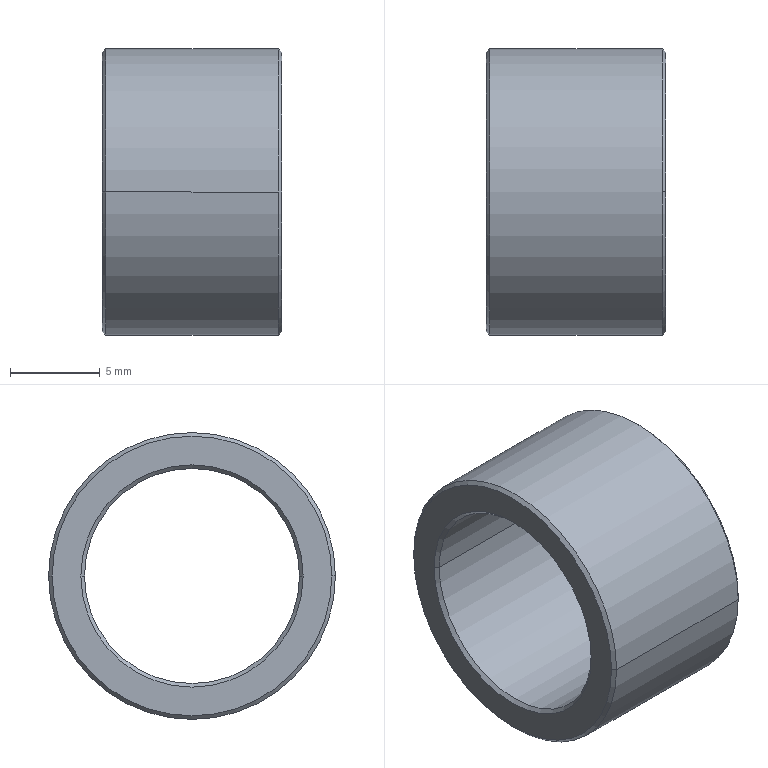Part | STEP file | 0230_009_KNCLB12-16-10 | 1 solid | 14 faces | box 10 x 16 x 16 mm | volume 876.127 mm3 | cone 8 | cylinder 4 | plane 2 | commonest cylinder face diameters 12 x2 16 x2
STEP:
#1=CARTESIAN_POINT('',(0.,0.,0.));
#2=DIRECTION('',(0.,0.,1.));
#3=DIRECTION('',(1.,0.,0.));
#4=AXIS2_PLACEMENT_3D('',#1,#2,#3);
#5=CARTESIAN_POINT('',(9.8,0.,8.));
#6=VERTEX_POINT('',#5);
#7=CARTESIAN_POINT('',(9.8,8.,0.));
#8=VERTEX_POINT('',#7);
#9=CARTESIAN_POINT('',(9.8,0.,0.));
#10=DIRECTION('',(-1.,0.,0.));
#11=DIRECTION('',(0.,-1.,0.));
#12=AXIS2_PLACEMENT_3D('',#9,#10,#11);
#13=CIRCLE('',#12,8.);
#14=CARTESIAN_POINT('',(5.,0.,0.));
#15=DIRECTION('',(-1.,0.,0.));
#16=DIRECTION('',(0.,-1.,0.));
#17=AXIS2_PLACEMENT_3D('',#14,#15,#16);
#18=CYLINDRICAL_SURFACE('',#17,8.);
#19=CARTESIAN_POINT('',(0.,-4.8));
#20=DIRECTION('',(1.,0.));
#21=VECTOR('',#20,1.);
#22=LINE('',#19,#21);
#23=(GEOMETRIC_REPRESENTATION_CONTEXT(2)PARAMETRIC_REPRESENTATION_CONTEXT()REPRESENTATION_CONTEXT('',''));
#24=DEFINITIONAL_REPRESENTATION('',(#22),#23);
#25=PCURVE('',#18,#24);
#26=CARTESIAN_POINT('',(9.8,0.,0.));
#27=DIRECTION('',(-1.,0.,0.));
#28=DIRECTION('',(0.,0.,1.));
#29=AXIS2_PLACEMENT_3D('',#26,#27,#28);
#30=CONICAL_SURFACE('',#29,8.,0.7854);
#31=CARTESIAN_POINT('',(-1.571,0.));
#32=DIRECTION('',(1.,0.));
#33=VECTOR('',#32,1.);
#34=LINE('',#31,#33);
#35=(GEOMETRIC_REPRESENTATION_CONTEXT(2)PARAMETRIC_REPRESENTATION_CONTEXT()REPRESENTATION_CONTEXT('',''));
#36=DEFINITIONAL_REPRESENTATION('',(#34),#35);
#37=PCURVE('',#30,#36);
#38=SURFACE_CURVE('',#13,(#25,#37),.PCURVE_S1.);
#39=EDGE_CURVE('',#6,#8,#38,.T.);
#40=ORIENTED_EDGE('',*,*,#39,.T.);
#41=CARTESIAN_POINT('',(0.2,8.,0.));
#42=VERTEX_POINT('',#41);
#43=CARTESIAN_POINT('',(5.,8.,0.));
#44=DIRECTION('',(-1.,0.,0.));
#45=VECTOR('',#44,1.);
#46=LINE('',#43,#45);
#47=CARTESIAN_POINT('',(3.142,0.));
#48=DIRECTION('',(0.,1.));
#49=VECTOR('',#48,1.);
#50=LINE('',#47,#49);
#51=(GEOMETRIC_REPRESENTATION_CONTEXT(2)PARAMETRIC_REPRESENTATION_CONTEXT()REPRESENTATION_CONTEXT('',''));
#52=DEFINITIONAL_REPRESENTATION('',(#50),#51);
#53=PCURVE('',#18,#52);
#54=CARTESIAN_POINT('',(5.,0.,0.));
#55=DIRECTION('',(-1.,0.,0.));
#56=DIRECTION('',(0.,-1.,0.));
#57=AXIS2_PLACEMENT_3D('',#54,#55,#56);
#58=CYLINDRICAL_SURFACE('',#57,8.);
#59=CARTESIAN_POINT('',(3.142,0.));
#60=DIRECTION('',(0.,1.));
#61=VECTOR('',#60,1.);
#62=LINE('',#59,#61);
#63=(GEOMETRIC_REPRESENTATION_CONTEXT(2)PARAMETRIC_REPRESENTATION_CONTEXT()REPRESENTATION_CONTEXT('',''));
#64=DEFINITIONAL_REPRESENTATION('',(#62),#63);
#65=PCURVE('',#58,#64);
#66=SURFACE_CURVE('',#46,(#53,#65),.PCURVE_S1.);
#67=EDGE_CURVE('',#8,#42,#66,.T.);
#68=ORIENTED_EDGE('',*,*,#67,.T.);
#69=CARTESIAN_POINT('',(0.2,-8.,0.));
#70=VERTEX_POINT('',#69);
#71=CARTESIAN_POINT('',(0.2,0.,0.));
#72=DIRECTION('',(1.,0.,0.));
#73=DIRECTION('',(0.,-1.,0.));
#74=AXIS2_PLACEMENT_3D('',#71,#72,#73);
#75=CIRCLE('',#74,8.);
#76=CARTESIAN_POINT('',(6.283,4.8));
#77=DIRECTION('',(-1.,0.));
#78=VECTOR('',#77,1.);
#79=LINE('',#76,#78);
#80=(GEOMETRIC_REPRESENTATION_CONTEXT(2)PARAMETRIC_REPRESENTATION_CONTEXT()REPRESENTATION_CONTEXT('',''));
#81=DEFINITIONAL_REPRESENTATION('',(#79),#80);
#82=PCURVE('',#18,#81);
#83=CARTESIAN_POINT('',(0.2,0.,0.));
#84=DIRECTION('',(1.,0.,0.));
#85=DIRECTION('',(0.,1.,0.));
#86=AXIS2_PLACEMENT_3D('',#83,#84,#85);
#87=CONICAL_SURFACE('',#86,8.,0.7854);
#88=CARTESIAN_POINT('',(-3.142,0.));
#89=DIRECTION('',(1.,0.));
#90=VECTOR('',#89,1.);
#91=LINE('',#88,#90);
#92=(GEOMETRIC_REPRESENTATION_CONTEXT(2)PARAMETRIC_REPRESENTATION_CONTEXT()REPRESENTATION_CONTEXT('',''));
#93=DEFINITIONAL_REPRESENTATION('',(#91),#92);
#94=PCURVE('',#87,#93);
#95=SURFACE_CURVE('',#75,(#82,#94),.PCURVE_S1.);
#96=EDGE_CURVE('',#42,#70,#95,.T.);
#97=ORIENTED_EDGE('',*,*,#96,.T.);
#98=CARTESIAN_POINT('',(9.8,-8.,0.));
#99=VERTEX_POINT('',#98);
#100=CARTESIAN_POINT('',(5.,-8.,0.));
#101=DIRECTION('',(-1.,0.,0.));
#102=VECTOR('',#101,1.);
#103=LINE('',#100,#102);
#104=CARTESIAN_POINT('',(0.,0.));
#105=DIRECTION('',(0.,1.));
#106=VECTOR('',#105,1.);
#107=LINE('',#104,#106);
#108=(GEOMETRIC_REPRESENTATION_CONTEXT(2)PARAMETRIC_REPRESENTATION_CONTEXT()REPRESENTATION_CONTEXT('',''));
#109=DEFINITIONAL_REPRESENTATION('',(#107),#108);
#110=PCURVE('',#18,#109);
#111=CARTESIAN_POINT('',(6.283,0.));
#112=DIRECTION('',(0.,1.));
#113=VECTOR('',#112,1.);
#114=LINE('',#111,#113);
#115=(GEOMETRIC_REPRESENTATION_CONTEXT(2)PARAMETRIC_REPRESENTATION_CONTEXT()REPRESENTATION_CONTEXT('',''));
#116=DEFINITIONAL_REPRESENTATION('',(#114),#115);
#117=PCURVE('',#58,#116);
#118=SURFACE_CURVE('',#103,(#110,#117),.PCURVE_S1.);
#119=EDGE_CURVE('',#99,#70,#118,.T.);
#120=ORIENTED_EDGE('',*,*,#119,.F.);
#121=CARTESIAN_POINT('',(9.8,0.,0.));
#122=DIRECTION('',(-1.,0.,0.));
#123=DIRECTION('',(0.,-1.,0.));
#124=AXIS2_PLACEMENT_3D('',#121,#122,#123);
#125=CIRCLE('',#124,8.);
#126=CARTESIAN_POINT('',(0.,-4.8));
#127=DIRECTION('',(1.,0.));
#128=VECTOR('',#127,1.);
#129=LINE('',#126,#128);
#130=(GEOMETRIC_REPRESENTATION_CONTEXT(2)PARAMETRIC_REPRESENTATION_CONTEXT()REPRESENTATION_CONTEXT('',''));
#131=DEFINITIONAL_REPRESENTATION('',(#129),#130);
#132=PCURVE('',#18,#131);
#133=CARTESIAN_POINT('',(9.8,0.,0.));
#134=DIRECTION('',(-1.,0.,0.));
#135=DIRECTION('',(0.,0.,1.));
#136=AXIS2_PLACEMENT_3D('',#133,#134,#135);
#137=CONICAL_SURFACE('',#136,8.,0.7854);
#138=CARTESIAN_POINT('',(4.712,0.));
#139=DIRECTION('',(1.,0.));
#140=VECTOR('',#139,1.);
#141=LINE('',#138,#140);
#142=(GEOMETRIC_REPRESENTATION_CONTEXT(2)PARAMETRIC_REPRESENTATION_CONTEXT()REPRESENTATION_CONTEXT('',''));
#143=DEFINITIONAL_REPRESENTATION('',(#141),#142);
#144=PCURVE('',#137,#143);
#145=SURFACE_CURVE('',#125,(#132,#144),.PCURVE_S1.);
#146=EDGE_CURVE('',#99,#6,#145,.T.);
#147=ORIENTED_EDGE('',*,*,#146,.T.);
#148=EDGE_LOOP('',(#40,#68,#97,#120,#147));
#149=FACE_BOUND('',#148,.T.);
#150=ADVANCED_FACE('',(#149),#18,.T.);
#151=CARTESIAN_POINT('',(10.,0.,7.8));
#152=VERTEX_POINT('',#151);
#153=CARTESIAN_POINT('',(10.,0.,-7.8));
#154=VERTEX_POINT('',#153);
#155=CARTESIAN_POINT('',(10.,0.,0.));
#156=DIRECTION('',(-1.,0.,0.));
#157=DIRECTION('',(0.,0.,1.));
#158=AXIS2_PLACEMENT_3D('',#155,#156,#157);
#159=CIRCLE('',#158,7.8);
#160=CARTESIAN_POINT('',(0.,-0.2));
#161=DIRECTION('',(1.,0.));
#162=VECTOR('',#161,1.);
#163=LINE('',#160,#162);
#164=(GEOMETRIC_REPRESENTATION_CONTEXT(2)PARAMETRIC_REPRESENTATION_CONTEXT()REPRESENTATION_CONTEXT('',''));
#165=DEFINITIONAL_REPRESENTATION('',(#163),#164);
#166=PCURVE('',#30,#165);
#167=CARTESIAN_POINT('',(10.,-7.,0.));
#168=DIRECTION('',(1.,0.,0.));
#169=DIRECTION('',(0.,0.,-1.));
#170=AXIS2_PLACEMENT_3D('',#167,#168,#169);
#171=PLANE('',#170);
#172=CARTESIAN_POINT('',(-7.8,7.));
#173=CARTESIAN_POINT('',(-7.8,20.51));
#174=CARTESIAN_POINT('',(3.9,13.755));
#175=CARTESIAN_POINT('',(15.6,7.));
#176=CARTESIAN_POINT('',(3.9,0.245));
#177=CARTESIAN_POINT('',(-7.8,-6.51));
#178=CARTESIAN_POINT('',(-7.8,7.));
#179=(BOUNDED_CURVE()B_SPLINE_CURVE(2,(#172,#173,#174,#175,#176,#177,#178),.UNSPECIFIED.,.T.,.F.)B_SPLINE_CURVE_WITH_KNOTS((1,2,2,2,2,1),(-2.094,0.,2.094,4.189,6.283,8.378),.UNSPECIFIED.)CURVE()GEOMETRIC_REPRESENTATION_ITEM()RATIONAL_B_SPLINE_CURVE((1.,0.5,1.,0.5,1.,0.5,1.))REPRESENTATION_ITEM(''));
#180=(GEOMETRIC_REPRESENTATION_CONTEXT(2)PARAMETRIC_REPRESENTATION_CONTEXT()REPRESENTATION_CONTEXT('',''));
#181=DEFINITIONAL_REPRESENTATION('',(#179),#180);
#182=PCURVE('',#171,#181);
#183=SURFACE_CURVE('',#159,(#166,#182),.PCURVE_S1.);
#184=EDGE_CURVE('',#152,#154,#183,.T.);
#185=ORIENTED_EDGE('',*,*,#184,.T.);
#186=CARTESIAN_POINT('',(9.8,0.,-8.));
#187=VERTEX_POINT('',#186);
#188=CARTESIAN_POINT('',(9.8,0.,-8.));
#189=DIRECTION('',(-0.7071,0.,-0.7071));
#190=VECTOR('',#189,1.);
#191=LINE('',#188,#190);
#192=CARTESIAN_POINT('',(3.142,0.));
#193=DIRECTION('',(0.,1.));
#194=VECTOR('',#193,1.);
#195=LINE('',#192,#194);
#196=(GEOMETRIC_REPRESENTATION_CONTEXT(2)PARAMETRIC_REPRESENTATION_CONTEXT()REPRESENTATION_CONTEXT('',''));
#197=DEFINITIONAL_REPRESENTATION('',(#195),#196);
#198=PCURVE('',#30,#197);
#199=CARTESIAN_POINT('',(3.142,0.));
#200=DIRECTION('',(0.,1.));
#201=VECTOR('',#200,1.);
#202=LINE('',#199,#201);
#203=(GEOMETRIC_REPRESENTATION_CONTEXT(2)PARAMETRIC_REPRESENTATION_CONTEXT()REPRESENTATION_CONTEXT('',''));
#204=DEFINITIONAL_REPRESENTATION('',(#202),#203);
#205=PCURVE('',#137,#204);
#206=SURFACE_CURVE('',#191,(#198,#205),.PCURVE_S1.);
#207=EDGE_CURVE('',#154,#187,#206,.T.);
#208=ORIENTED_EDGE('',*,*,#207,.T.);
#209=CARTESIAN_POINT('',(9.8,0.,0.));
#210=DIRECTION('',(-1.,0.,0.));
#211=DIRECTION('',(0.,-1.,0.));
#212=AXIS2_PLACEMENT_3D('',#209,#210,#211);
#213=CIRCLE('',#212,8.);
#214=CARTESIAN_POINT('',(-1.571,0.));
#215=DIRECTION('',(1.,0.));
#216=VECTOR('',#215,1.);
#217=LINE('',#214,#216);
#218=(GEOMETRIC_REPRESENTATION_CONTEXT(2)PARAMETRIC_REPRESENTATION_CONTEXT()REPRESENTATION_CONTEXT('',''));
#219=DEFINITIONAL_REPRESENTATION('',(#217),#218);
#220=PCURVE('',#30,#219);
#221=CARTESIAN_POINT('',(0.,-4.8));
#222=DIRECTION('',(1.,0.));
#223=VECTOR('',#222,1.);
#224=LINE('',#221,#223);
#225=(GEOMETRIC_REPRESENTATION_CONTEXT(2)PARAMETRIC_REPRESENTATION_CONTEXT()REPRESENTATION_CONTEXT('',''));
#226=DEFINITIONAL_REPRESENTATION('',(#224),#225);
#227=PCURVE('',#58,#226);
#228=SURFACE_CURVE('',#213,(#220,#227),.PCURVE_S1.);
#229=EDGE_CURVE('',#8,#187,#228,.T.);
#230=ORIENTED_EDGE('',*,*,#229,.F.);
#231=ORIENTED_EDGE('',*,*,#39,.F.);
#232=CARTESIAN_POINT('',(9.8,0.,8.));
#233=DIRECTION('',(-0.7071,0.,0.7071));
#234=VECTOR('',#233,1.);
#235=LINE('',#232,#234);
#236=CARTESIAN_POINT('',(0.,0.));
#237=DIRECTION('',(0.,1.));
#238=VECTOR('',#237,1.);
#239=LINE('',#236,#238);
#240=(GEOMETRIC_REPRESENTATION_CONTEXT(2)PARAMETRIC_REPRESENTATION_CONTEXT()REPRESENTATION_CONTEXT('',''));
#241=DEFINITIONAL_REPRESENTATION('',(#239),#240);
#242=PCURVE('',#30,#241);
#243=CARTESIAN_POINT('',(6.283,0.));
#244=DIRECTION('',(0.,1.));
#245=VECTOR('',#244,1.);
#246=LINE('',#243,#245);
#247=(GEOMETRIC_REPRESENTATION_CONTEXT(2)PARAMETRIC_REPRESENTATION_CONTEXT()REPRESENTATION_CONTEXT('',''));
#248=DEFINITIONAL_REPRESENTATION('',(#246),#247);
#249=PCURVE('',#137,#248);
#250=SURFACE_CURVE('',#235,(#242,#249),.PCURVE_S1.);
#251=EDGE_CURVE('',#152,#6,#250,.T.);
#252=ORIENTED_EDGE('',*,*,#251,.F.);
#253=EDGE_LOOP('',(#185,#208,#230,#231,#252));
#254=FACE_BOUND('',#253,.T.);
#255=ADVANCED_FACE('',(#254),#30,.T.);
#256=CARTESIAN_POINT('',(0.,7.8,0.));
#257=VERTEX_POINT('',#256);
#258=CARTESIAN_POINT('',(0.,-7.8,0.));
#259=VERTEX_POINT('',#258);
#260=CARTESIAN_POINT('',(0.,0.,0.));
#261=DIRECTION('',(1.,0.,0.));
#262=DIRECTION('',(0.,1.,0.));
#263=AXIS2_PLACEMENT_3D('',#260,#261,#262);
#264=CIRCLE('',#263,7.8);
#265=CARTESIAN_POINT('',(0.,-0.2));
#266=DIRECTION('',(1.,0.));
#267=VECTOR('',#266,1.);
#268=LINE('',#265,#267);
#269=(GEOMETRIC_REPRESENTATION_CONTEXT(2)PARAMETRIC_REPRESENTATION_CONTEXT()REPRESENTATION_CONTEXT('',''));
#270=DEFINITIONAL_REPRESENTATION('',(#268),#269);
#271=PCURVE('',#87,#270);
#272=CARTESIAN_POINT('',(0.,-7.,0.));
#273=DIRECTION('',(-1.,0.,0.));
#274=DIRECTION('',(0.,-1.,0.));
#275=AXIS2_PLACEMENT_3D('',#272,#273,#274);
#276=PLANE('',#275);
#277=CARTESIAN_POINT('',(-14.8,0.));
#278=CARTESIAN_POINT('',(-14.8,13.51));
#279=CARTESIAN_POINT('',(-3.1,6.755));
#280=CARTESIAN_POINT('',(8.6,0.));
#281=CARTESIAN_POINT('',(-3.1,-6.755));
#282=CARTESIAN_POINT('',(-14.8,-13.51));
#283=CARTESIAN_POINT('',(-14.8,0.));
#284=(BOUNDED_CURVE()B_SPLINE_CURVE(2,(#277,#278,#279,#280,#281,#282,#283),.UNSPECIFIED.,.T.,.F.)B_SPLINE_CURVE_WITH_KNOTS((1,2,2,2,2,1),(-2.094,0.,2.094,4.189,6.283,8.378),.UNSPECIFIED.)CURVE()GEOMETRIC_REPRESENTATION_ITEM()RATIONAL_B_SPLINE_CURVE((1.,0.5,1.,0.5,1.,0.5,1.))REPRESENTATION_ITEM(''));
#285=(GEOMETRIC_REPRESENTATION_CONTEXT(2)PARAMETRIC_REPRESENTATION_CONTEXT()REPRESENTATION_CONTEXT('',''));
#286=DEFINITIONAL_REPRESENTATION('',(#284),#285);
#287=PCURVE('',#276,#286);
#288=SURFACE_CURVE('',#264,(#271,#287),.PCURVE_S1.);
#289=EDGE_CURVE('',#257,#259,#288,.T.);
#290=ORIENTED_EDGE('',*,*,#289,.T.);
#291=CARTESIAN_POINT('',(0.2,-8.,0.));
#292=DIRECTION('',(0.7071,-0.7071,0.));
#293=VECTOR('',#292,1.);
#294=LINE('',#291,#293);
#295=CARTESIAN_POINT('',(3.142,0.));
#296=DIRECTION('',(0.,1.));
#297=VECTOR('',#296,1.);
#298=LINE('',#295,#297);
#299=(GEOMETRIC_REPRESENTATION_CONTEXT(2)PARAMETRIC_REPRESENTATION_CONTEXT()REPRESENTATION_CONTEXT('',''));
#300=DEFINITIONAL_REPRESENTATION('',(#298),#299);
#301=PCURVE('',#87,#300);
#302=CARTESIAN_POINT('',(0.2,0.,0.));
#303=DIRECTION('',(1.,0.,0.));
#304=DIRECTION('',(0.,1.,0.));
#305=AXIS2_PLACEMENT_3D('',#302,#303,#304);
#306=CONICAL_SURFACE('',#305,8.,0.7854);
#307=CARTESIAN_POINT('',(3.142,0.));
#308=DIRECTION('',(0.,1.));
#309=VECTOR('',#308,1.);
#310=LINE('',#307,#309);
#311=(GEOMETRIC_REPRESENTATION_CONTEXT(2)PARAMETRIC_REPRESENTATION_CONTEXT()REPRESENTATION_CONTEXT('',''));
#312=DEFINITIONAL_REPRESENTATION('',(#310),#311);
#313=PCURVE('',#306,#312);
#314=SURFACE_CURVE('',#294,(#301,#313),.PCURVE_S1.);
#315=EDGE_CURVE('',#259,#70,#314,.T.);
#316=ORIENTED_EDGE('',*,*,#315,.T.);
#317=ORIENTED_EDGE('',*,*,#96,.F.);
#318=CARTESIAN_POINT('',(0.2,8.,0.));
#319=DIRECTION('',(0.7071,0.7071,0.));
#320=VECTOR('',#319,1.);
#321=LINE('',#318,#320);
#322=CARTESIAN_POINT('',(0.,0.));
#323=DIRECTION('',(0.,1.));
#324=VECTOR('',#323,1.);
#325=LINE('',#322,#324);
#326=(GEOMETRIC_REPRESENTATION_CONTEXT(2)PARAMETRIC_REPRESENTATION_CONTEXT()REPRESENTATION_CONTEXT('',''));
#327=DEFINITIONAL_REPRESENTATION('',(#325),#326);
#328=PCURVE('',#87,#327);
#329=CARTESIAN_POINT('',(6.283,0.));
#330=DIRECTION('',(0.,1.));
#331=VECTOR('',#330,1.);
#332=LINE('',#329,#331);
#333=(GEOMETRIC_REPRESENTATION_CONTEXT(2)PARAMETRIC_REPRESENTATION_CONTEXT()REPRESENTATION_CONTEXT('',''));
#334=DEFINITIONAL_REPRESENTATION('',(#332),#333);
#335=PCURVE('',#306,#334);
#336=SURFACE_CURVE('',#321,(#328,#335),.PCURVE_S1.);
#337=EDGE_CURVE('',#257,#42,#336,.T.);
#338=ORIENTED_EDGE('',*,*,#337,.F.);
#339=EDGE_LOOP('',(#290,#316,#317,#338));
#340=FACE_BOUND('',#339,.T.);
#341=ADVANCED_FACE('',(#340),#87,.T.);
#342=CARTESIAN_POINT('',(9.8,-6.,0.));
#343=VERTEX_POINT('',#342);
#344=CARTESIAN_POINT('',(9.8,0.,-6.));
#345=VERTEX_POINT('',#344);
#346=CARTESIAN_POINT('',(9.8,0.,0.));
#347=DIRECTION('',(1.,0.,0.));
#348=DIRECTION('',(0.,-1.,0.));
#349=AXIS2_PLACEMENT_3D('',#346,#347,#348);
#350=CIRCLE('',#349,6.);
#351=CARTESIAN_POINT('',(10.,0.,0.));
#352=DIRECTION('',(1.,0.,0.));
#353=DIRECTION('',(0.,0.,-1.));
#354=AXIS2_PLACEMENT_3D('',#351,#352,#353);
#355=CONICAL_SURFACE('',#354,6.2,0.7854);
#356=CARTESIAN_POINT('',(4.712,-0.2));
#357=DIRECTION('',(1.,0.));
#358=VECTOR('',#357,1.);
#359=LINE('',#356,#358);
#360=(GEOMETRIC_REPRESENTATION_CONTEXT(2)PARAMETRIC_REPRESENTATION_CONTEXT()REPRESENTATION_CONTEXT('',''));
#361=DEFINITIONAL_REPRESENTATION('',(#359),#360);
#362=PCURVE('',#355,#361);
#363=CARTESIAN_POINT('',(5.,0.,0.));
#364=DIRECTION('',(-1.,0.,0.));
#365=DIRECTION('',(0.,-1.,0.));
#366=AXIS2_PLACEMENT_3D('',#363,#364,#365);
#367=CYLINDRICAL_SURFACE('',#366,6.);
#368=CARTESIAN_POINT('',(6.283,-4.8));
#369=DIRECTION('',(-1.,0.));
#370=VECTOR('',#369,1.);
#371=LINE('',#368,#370);
#372=(GEOMETRIC_REPRESENTATION_CONTEXT(2)PARAMETRIC_REPRESENTATION_CONTEXT()REPRESENTATION_CONTEXT('',''));
#373=DEFINITIONAL_REPRESENTATION('',(#371),#372);
#374=PCURVE('',#367,#373);
#375=SURFACE_CURVE('',#350,(#362,#374),.PCURVE_S1.);
#376=EDGE_CURVE('',#343,#345,#375,.T.);
#377=ORIENTED_EDGE('',*,*,#376,.T.);
#378=CARTESIAN_POINT('',(10.,0.,-6.2));
#379=VERTEX_POINT('',#378);
#380=CARTESIAN_POINT('',(10.,0.,-6.2));
#381=DIRECTION('',(0.7071,0.,-0.7071));
#382=VECTOR('',#381,1.);
#383=LINE('',#380,#382);
#384=CARTESIAN_POINT('',(6.283,0.));
#385=DIRECTION('',(0.,1.));
#386=VECTOR('',#385,1.);
#387=LINE('',#384,#386);
#388=(GEOMETRIC_REPRESENTATION_CONTEXT(2)PARAMETRIC_REPRESENTATION_CONTEXT()REPRESENTATION_CONTEXT('',''));
#389=DEFINITIONAL_REPRESENTATION('',(#387),#388);
#390=PCURVE('',#355,#389);
#391=CARTESIAN_POINT('',(10.,0.,0.));
#392=DIRECTION('',(1.,0.,0.));
#393=DIRECTION('',(0.,0.,-1.));
#394=AXIS2_PLACEMENT_3D('',#391,#392,#393);
#395=CONICAL_SURFACE('',#394,6.2,0.7854);
#396=CARTESIAN_POINT('',(0.,0.));
#397=DIRECTION('',(0.,1.));
#398=VECTOR('',#397,1.);
#399=LINE('',#396,#398);
#400=(GEOMETRIC_REPRESENTATION_CONTEXT(2)PARAMETRIC_REPRESENTATION_CONTEXT()REPRESENTATION_CONTEXT('',''));
#401=DEFINITIONAL_REPRESENTATION('',(#399),#400);
#402=PCURVE('',#395,#401);
#403=SURFACE_CURVE('',#383,(#390,#402),.PCURVE_S1.);
#404=EDGE_CURVE('',#345,#379,#403,.T.);
#405=ORIENTED_EDGE('',*,*,#404,.T.);
#406=CARTESIAN_POINT('',(10.,0.,6.2));
#407=VERTEX_POINT('',#406);
#408=CARTESIAN_POINT('',(10.,0.,0.));
#409=DIRECTION('',(-1.,0.,0.));
#410=DIRECTION('',(0.,0.,-1.));
#411=AXIS2_PLACEMENT_3D('',#408,#409,#410);
#412=CIRCLE('',#411,6.2);
#413=CARTESIAN_POINT('',(6.283,0.));
#414=DIRECTION('',(-1.,0.));
#415=VECTOR('',#414,1.);
#416=LINE('',#413,#415);
#417=(GEOMETRIC_REPRESENTATION_CONTEXT(2)PARAMETRIC_REPRESENTATION_CONTEXT()REPRESENTATION_CONTEXT('',''));
#418=DEFINITIONAL_REPRESENTATION('',(#416),#417);
#419=PCURVE('',#355,#418);
#420=CARTESIAN_POINT('',(6.2,7.));
#421=CARTESIAN_POINT('',(6.2,-3.739));
#422=CARTESIAN_POINT('',(-3.1,1.631));
#423=CARTESIAN_POINT('',(-12.4,7.));
#424=CARTESIAN_POINT('',(-3.1,12.369));
#425=CARTESIAN_POINT('',(6.2,17.739));
#426=CARTESIAN_POINT('',(6.2,7.));
#427=(BOUNDED_CURVE()B_SPLINE_CURVE(2,(#420,#421,#422,#423,#424,#425,#426),.UNSPECIFIED.,.T.,.F.)B_SPLINE_CURVE_WITH_KNOTS((1,2,2,2,2,1),(-2.094,0.,2.094,4.189,6.283,8.378),.UNSPECIFIED.)CURVE()GEOMETRIC_REPRESENTATION_ITEM()RATIONAL_B_SPLINE_CURVE((1.,0.5,1.,0.5,1.,0.5,1.))REPRESENTATION_ITEM(''));
#428=(GEOMETRIC_REPRESENTATION_CONTEXT(2)PARAMETRIC_REPRESENTATION_CONTEXT()REPRESENTATION_CONTEXT('',''));
#429=DEFINITIONAL_REPRESENTATION('',(#427),#428);
#430=PCURVE('',#171,#429);
#431=SURFACE_CURVE('',#412,(#419,#430),.PCURVE_S1.);
#432=EDGE_CURVE('',#379,#407,#431,.T.);
#433=ORIENTED_EDGE('',*,*,#432,.T.);
#434=CARTESIAN_POINT('',(9.8,0.,6.));
#435=VERTEX_POINT('',#434);
#436=CARTESIAN_POINT('',(10.,0.,6.2));
#437=DIRECTION('',(0.7071,0.,0.7071));
#438=VECTOR('',#437,1.);
#439=LINE('',#436,#438);
#440=CARTESIAN_POINT('',(3.142,0.));
#441=DIRECTION('',(0.,1.));
#442=VECTOR('',#441,1.);
#443=LINE('',#440,#442);
#444=(GEOMETRIC_REPRESENTATION_CONTEXT(2)PARAMETRIC_REPRESENTATION_CONTEXT()REPRESENTATION_CONTEXT('',''));
#445=DEFINITIONAL_REPRESENTATION('',(#443),#444);
#446=PCURVE('',#355,#445);
#447=CARTESIAN_POINT('',(3.142,0.));
#448=DIRECTION('',(0.,1.));
#449=VECTOR('',#448,1.);
#450=LINE('',#447,#449);
#451=(GEOMETRIC_REPRESENTATION_CONTEXT(2)PARAMETRIC_REPRESENTATION_CONTEXT()REPRESENTATION_CONTEXT('',''));
#452=DEFINITIONAL_REPRESENTATION('',(#450),#451);
#453=PCURVE('',#395,#452);
#454=SURFACE_CURVE('',#439,(#446,#453),.PCURVE_S1.);
#455=EDGE_CURVE('',#435,#407,#454,.T.);
#456=ORIENTED_EDGE('',*,*,#455,.F.);
#457=CARTESIAN_POINT('',(9.8,0.,0.));
#458=DIRECTION('',(1.,0.,0.));
#459=DIRECTION('',(0.,-1.,0.));
#460=AXIS2_PLACEMENT_3D('',#457,#458,#459);
#461=CIRCLE('',#460,6.);
#462=CARTESIAN_POINT('',(-1.571,-0.2));
#463=DIRECTION('',(1.,0.));
#464=VECTOR('',#463,1.);
#465=LINE('',#462,#464);
#466=(GEOMETRIC_REPRESENTATION_CONTEXT(2)PARAMETRIC_REPRESENTATION_CONTEXT()REPRESENTATION_CONTEXT('',''));
#467=DEFINITIONAL_REPRESENTATION('',(#465),#466);
#468=PCURVE('',#355,#467);
#469=CARTESIAN_POINT('',(5.,0.,0.));
#470=DIRECTION('',(-1.,0.,0.));
#471=DIRECTION('',(0.,-1.,0.));
#472=AXIS2_PLACEMENT_3D('',#469,#470,#471);
#473=CYLINDRICAL_SURFACE('',#472,6.);
#474=CARTESIAN_POINT('',(6.283,-4.8));
#475=DIRECTION('',(-1.,0.));
#476=VECTOR('',#475,1.);
#477=LINE('',#474,#476);
#478=(GEOMETRIC_REPRESENTATION_CONTEXT(2)PARAMETRIC_REPRESENTATION_CONTEXT()REPRESENTATION_CONTEXT('',''));
#479=DEFINITIONAL_REPRESENTATION('',(#477),#478);
#480=PCURVE('',#473,#479);
#481=SURFACE_CURVE('',#461,(#468,#480),.PCURVE_S1.);
#482=EDGE_CURVE('',#435,#343,#481,.T.);
#483=ORIENTED_EDGE('',*,*,#482,.T.);
#484=EDGE_LOOP('',(#377,#405,#433,#456,#483));
#485=FACE_BOUND('',#484,.F.);
#486=ADVANCED_FACE('',(#485),#355,.F.);
#487=CARTESIAN_POINT('',(0.2,-6.,0.));
#488=VERTEX_POINT('',#487);
#489=CARTESIAN_POINT('',(0.,-6.2,0.));
#490=VERTEX_POINT('',#489);
#491=CARTESIAN_POINT('',(0.,-6.2,0.));
#492=DIRECTION('',(-0.7071,-0.7071,0.));
#493=VECTOR('',#492,1.);
#494=LINE('',#491,#493);
#495=CARTESIAN_POINT('',(0.,0.,0.));
#496=DIRECTION('',(-1.,0.,0.));
#497=DIRECTION('',(0.,-1.,0.));
#498=AXIS2_PLACEMENT_3D('',#495,#496,#497);
#499=CONICAL_SURFACE('',#498,6.2,0.7854);
#500=CARTESIAN_POINT('',(6.283,0.));
#501=DIRECTION('',(0.,1.));
#502=VECTOR('',#501,1.);
#503=LINE('',#500,#502);
#504=(GEOMETRIC_REPRESENTATION_CONTEXT(2)PARAMETRIC_REPRESENTATION_CONTEXT()REPRESENTATION_CONTEXT('',''));
#505=DEFINITIONAL_REPRESENTATION('',(#503),#504);
#506=PCURVE('',#499,#505);
#507=CARTESIAN_POINT('',(0.,0.,0.));
#508=DIRECTION('',(-1.,0.,0.));
#509=DIRECTION('',(0.,-1.,0.));
#510=AXIS2_PLACEMENT_3D('',#507,#508,#509);
#511=CONICAL_SURFACE('',#510,6.2,0.7854);
#512=CARTESIAN_POINT('',(0.,0.));
#513=DIRECTION('',(0.,1.));
#514=VECTOR('',#513,1.);
#515=LINE('',#512,#514);
#516=(GEOMETRIC_REPRESENTATION_CONTEXT(2)PARAMETRIC_REPRESENTATION_CONTEXT()REPRESENTATION_CONTEXT('',''));
#517=DEFINITIONAL_REPRESENTATION('',(#515),#516);
#518=PCURVE('',#511,#517);
#519=SURFACE_CURVE('',#494,(#506,#518),.PCURVE_S1.);
#520=EDGE_CURVE('',#488,#490,#519,.T.);
#521=ORIENTED_EDGE('',*,*,#520,.T.);
#522=CARTESIAN_POINT('',(0.,6.2,0.));
#523=VERTEX_POINT('',#522);
#524=CARTESIAN_POINT('',(0.,0.,0.));
#525=DIRECTION('',(1.,0.,0.));
#526=DIRECTION('',(0.,-1.,0.));
#527=AXIS2_PLACEMENT_3D('',#524,#525,#526);
#528=CIRCLE('',#527,6.2);
#529=CARTESIAN_POINT('',(6.283,0.));
#530=DIRECTION('',(-1.,0.));
#531=VECTOR('',#530,1.);
#532=LINE('',#529,#531);
#533=(GEOMETRIC_REPRESENTATION_CONTEXT(2)PARAMETRIC_REPRESENTATION_CONTEXT()REPRESENTATION_CONTEXT('',''));
#534=DEFINITIONAL_REPRESENTATION('',(#532),#533);
#535=PCURVE('',#499,#534);
#536=CARTESIAN_POINT('',(-0.8,0.));
#537=CARTESIAN_POINT('',(-0.8,-10.739));
#538=CARTESIAN_POINT('',(-10.1,-5.369));
#539=CARTESIAN_POINT('',(-19.4,0.));
#540=CARTESIAN_POINT('',(-10.1,5.369));
#541=CARTESIAN_POINT('',(-0.8,10.739));
#542=CARTESIAN_POINT('',(-0.8,0.));
#543=(BOUNDED_CURVE()B_SPLINE_CURVE(2,(#536,#537,#538,#539,#540,#541,#542),.UNSPECIFIED.,.T.,.F.)B_SPLINE_CURVE_WITH_KNOTS((1,2,2,2,2,1),(-2.094,0.,2.094,4.189,6.283,8.378),.UNSPECIFIED.)CURVE()GEOMETRIC_REPRESENTATION_ITEM()RATIONAL_B_SPLINE_CURVE((1.,0.5,1.,0.5,1.,0.5,1.))REPRESENTATION_ITEM(''));
#544=(GEOMETRIC_REPRESENTATION_CONTEXT(2)PARAMETRIC_REPRESENTATION_CONTEXT()REPRESENTATION_CONTEXT('',''));
#545=DEFINITIONAL_REPRESENTATION('',(#543),#544);
#546=PCURVE('',#276,#545);
#547=SURFACE_CURVE('',#528,(#535,#546),.PCURVE_S1.);
#548=EDGE_CURVE('',#490,#523,#547,.T.);
#549=ORIENTED_EDGE('',*,*,#548,.T.);
#550=CARTESIAN_POINT('',(0.2,6.,0.));
#551=VERTEX_POINT('',#550);
#552=CARTESIAN_POINT('',(0.,6.2,0.));
#553=DIRECTION('',(-0.7071,0.7071,0.));
#554=VECTOR('',#553,1.);
#555=LINE('',#552,#554);
#556=CARTESIAN_POINT('',(3.142,0.));
#557=DIRECTION('',(0.,1.));
#558=VECTOR('',#557,1.);
#559=LINE('',#556,#558);
#560=(GEOMETRIC_REPRESENTATION_CONTEXT(2)PARAMETRIC_REPRESENTATION_CONTEXT()REPRESENTATION_CONTEXT('',''));
#561=DEFINITIONAL_REPRESENTATION('',(#559),#560);
#562=PCURVE('',#499,#561);
#563=CARTESIAN_POINT('',(3.142,0.));
#564=DIRECTION('',(0.,1.));
#565=VECTOR('',#564,1.);
#566=LINE('',#563,#565);
#567=(GEOMETRIC_REPRESENTATION_CONTEXT(2)PARAMETRIC_REPRESENTATION_CONTEXT()REPRESENTATION_CONTEXT('',''));
#568=DEFINITIONAL_REPRESENTATION('',(#566),#567);
#569=PCURVE('',#511,#568);
#570=SURFACE_CURVE('',#555,(#562,#569),.PCURVE_S1.);
#571=EDGE_CURVE('',#551,#523,#570,.T.);
#572=ORIENTED_EDGE('',*,*,#571,.F.);
#573=CARTESIAN_POINT('',(0.2,0.,0.));
#574=DIRECTION('',(-1.,0.,0.));
#575=DIRECTION('',(0.,-1.,0.));
#576=AXIS2_PLACEMENT_3D('',#573,#574,#575);
#577=CIRCLE('',#576,6.);
#578=CARTESIAN_POINT('',(0.,-0.2));
#579=DIRECTION('',(1.,0.));
#580=VECTOR('',#579,1.);
#581=LINE('',#578,#580);
#582=(GEOMETRIC_REPRESENTATION_CONTEXT(2)PARAMETRIC_REPRESENTATION_CONTEXT()REPRESENTATION_CONTEXT('',''));
#583=DEFINITIONAL_REPRESENTATION('',(#581),#582);
#584=PCURVE('',#499,#583);
#585=CARTESIAN_POINT('',(0.,4.8));
#586=DIRECTION('',(1.,0.));
#587=VECTOR('',#586,1.);
#588=LINE('',#585,#587);
#589=(GEOMETRIC_REPRESENTATION_CONTEXT(2)PARAMETRIC_REPRESENTATION_CONTEXT()REPRESENTATION_CONTEXT('',''));
#590=DEFINITIONAL_REPRESENTATION('',(#588),#589);
#591=PCURVE('',#367,#590);
#592=SURFACE_CURVE('',#577,(#584,#591),.PCURVE_S1.);
#593=EDGE_CURVE('',#551,#488,#592,.T.);
#594=ORIENTED_EDGE('',*,*,#593,.T.);
#595=EDGE_LOOP('',(#521,#549,#572,#594));
#596=FACE_BOUND('',#595,.F.);
#597=ADVANCED_FACE('',(#596),#499,.F.);
#598=CARTESIAN_POINT('',(5.,-6.,0.));
#599=DIRECTION('',(-1.,0.,0.));
#600=VECTOR('',#599,1.);
#601=LINE('',#598,#600);
#602=CARTESIAN_POINT('',(6.283,0.));
#603=DIRECTION('',(0.,1.));
#604=VECTOR('',#603,1.);
#605=LINE('',#602,#604);
#606=(GEOMETRIC_REPRESENTATION_CONTEXT(2)PARAMETRIC_REPRESENTATION_CONTEXT()REPRESENTATION_CONTEXT('',''));
#607=DEFINITIONAL_REPRESENTATION('',(#605),#606);
#608=PCURVE('',#367,#607);
#609=CARTESIAN_POINT('',(0.,0.));
#610=DIRECTION('',(0.,1.));
#611=VECTOR('',#610,1.);
#612=LINE('',#609,#611);
#613=(GEOMETRIC_REPRESENTATION_CONTEXT(2)PARAMETRIC_REPRESENTATION_CONTEXT()REPRESENTATION_CONTEXT('',''));
#614=DEFINITIONAL_REPRESENTATION('',(#612),#613);
#615=PCURVE('',#473,#614);
#616=SURFACE_CURVE('',#601,(#608,#615),.PCURVE_S1.);
#617=EDGE_CURVE('',#343,#488,#616,.T.);
#618=ORIENTED_EDGE('',*,*,#617,.T.);
#619=ORIENTED_EDGE('',*,*,#593,.F.);
#620=CARTESIAN_POINT('',(9.8,6.,0.));
#621=VERTEX_POINT('',#620);
#622=CARTESIAN_POINT('',(5.,6.,0.));
#623=DIRECTION('',(-1.,0.,0.));
#624=VECTOR('',#623,1.);
#625=LINE('',#622,#624);
#626=CARTESIAN_POINT('',(3.142,0.));
#627=DIRECTION('',(0.,1.));
#628=VECTOR('',#627,1.);
#629=LINE('',#626,#628);
#630=(GEOMETRIC_REPRESENTATION_CONTEXT(2)PARAMETRIC_REPRESENTATION_CONTEXT()REPRESENTATION_CONTEXT('',''));
#631=DEFINITIONAL_REPRESENTATION('',(#629),#630);
#632=PCURVE('',#367,#631);
#633=CARTESIAN_POINT('',(3.142,0.));
#634=DIRECTION('',(0.,1.));
#635=VECTOR('',#634,1.);
#636=LINE('',#633,#635);
#637=(GEOMETRIC_REPRESENTATION_CONTEXT(2)PARAMETRIC_REPRESENTATION_CONTEXT()REPRESENTATION_CONTEXT('',''));
#638=DEFINITIONAL_REPRESENTATION('',(#636),#637);
#639=PCURVE('',#473,#638);
#640=SURFACE_CURVE('',#625,(#632,#639),.PCURVE_S1.);
#641=EDGE_CURVE('',#621,#551,#640,.T.);
#642=ORIENTED_EDGE('',*,*,#641,.F.);
#643=CARTESIAN_POINT('',(9.8,0.,0.));
#644=DIRECTION('',(1.,0.,0.));
#645=DIRECTION('',(0.,-1.,0.));
#646=AXIS2_PLACEMENT_3D('',#643,#644,#645);
#647=CIRCLE('',#646,6.);
#648=CARTESIAN_POINT('',(6.283,-4.8));
#649=DIRECTION('',(-1.,0.));
#650=VECTOR('',#649,1.);
#651=LINE('',#648,#650);
#652=(GEOMETRIC_REPRESENTATION_CONTEXT(2)PARAMETRIC_REPRESENTATION_CONTEXT()REPRESENTATION_CONTEXT('',''));
#653=DEFINITIONAL_REPRESENTATION('',(#651),#652);
#654=PCURVE('',#367,#653);
#655=CARTESIAN_POINT('',(-1.571,-0.2));
#656=DIRECTION('',(1.,0.));
#657=VECTOR('',#656,1.);
#658=LINE('',#655,#657);
#659=(GEOMETRIC_REPRESENTATION_CONTEXT(2)PARAMETRIC_REPRESENTATION_CONTEXT()REPRESENTATION_CONTEXT('',''));
#660=DEFINITIONAL_REPRESENTATION('',(#658),#659);
#661=PCURVE('',#395,#660);
#662=SURFACE_CURVE('',#647,(#654,#661),.PCURVE_S1.);
#663=EDGE_CURVE('',#345,#621,#662,.T.);
#664=ORIENTED_EDGE('',*,*,#663,.F.);
#665=ORIENTED_EDGE('',*,*,#376,.F.);
#666=EDGE_LOOP('',(#618,#619,#642,#664,#665));
#667=FACE_BOUND('',#666,.F.);
#668=ADVANCED_FACE('',(#667),#367,.F.);
#669=ORIENTED_EDGE('',*,*,#67,.F.);
#670=ORIENTED_EDGE('',*,*,#229,.T.);
#671=CARTESIAN_POINT('',(9.8,0.,0.));
#672=DIRECTION('',(-1.,0.,0.));
#673=DIRECTION('',(0.,-1.,0.));
#674=AXIS2_PLACEMENT_3D('',#671,#672,#673);
#675=CIRCLE('',#674,8.);
#676=CARTESIAN_POINT('',(0.,-4.8));
#677=DIRECTION('',(1.,0.));
#678=VECTOR('',#677,1.);
#679=LINE('',#676,#678);
#680=(GEOMETRIC_REPRESENTATION_CONTEXT(2)PARAMETRIC_REPRESENTATION_CONTEXT()REPRESENTATION_CONTEXT('',''));
#681=DEFINITIONAL_REPRESENTATION('',(#679),#680);
#682=PCURVE('',#58,#681);
#683=CARTESIAN_POINT('',(-1.571,0.));
#684=DIRECTION('',(1.,0.));
#685=VECTOR('',#684,1.);
#686=LINE('',#683,#685);
#687=(GEOMETRIC_REPRESENTATION_CONTEXT(2)PARAMETRIC_REPRESENTATION_CONTEXT()REPRESENTATION_CONTEXT('',''));
#688=DEFINITIONAL_REPRESENTATION('',(#686),#687);
#689=PCURVE('',#137,#688);
#690=SURFACE_CURVE('',#675,(#682,#689),.PCURVE_S1.);
#691=EDGE_CURVE('',#187,#99,#690,.T.);
#692=ORIENTED_EDGE('',*,*,#691,.T.);
#693=ORIENTED_EDGE('',*,*,#119,.T.);
#694=CARTESIAN_POINT('',(0.2,0.,0.));
#695=DIRECTION('',(1.,0.,0.));
#696=DIRECTION('',(0.,-1.,0.));
#697=AXIS2_PLACEMENT_3D('',#694,#695,#696);
#698=CIRCLE('',#697,8.);
#699=CARTESIAN_POINT('',(6.283,4.8));
#700=DIRECTION('',(-1.,0.));
#701=VECTOR('',#700,1.);
#702=LINE('',#699,#701);
#703=(GEOMETRIC_REPRESENTATION_CONTEXT(2)PARAMETRIC_REPRESENTATION_CONTEXT()REPRESENTATION_CONTEXT('',''));
#704=DEFINITIONAL_REPRESENTATION('',(#702),#703);
#705=PCURVE('',#58,#704);
#706=CARTESIAN_POINT('',(3.142,0.));
#707=DIRECTION('',(1.,0.));
#708=VECTOR('',#707,1.);
#709=LINE('',#706,#708);
#710=(GEOMETRIC_REPRESENTATION_CONTEXT(2)PARAMETRIC_REPRESENTATION_CONTEXT()REPRESENTATION_CONTEXT('',''));
#711=DEFINITIONAL_REPRESENTATION('',(#709),#710);
#712=PCURVE('',#306,#711);
#713=SURFACE_CURVE('',#698,(#705,#712),.PCURVE_S1.);
#714=EDGE_CURVE('',#70,#42,#713,.T.);
#715=ORIENTED_EDGE('',*,*,#714,.T.);
#716=EDGE_LOOP('',(#669,#670,#692,#693,#715));
#717=FACE_BOUND('',#716,.T.);
#718=ADVANCED_FACE('',(#717),#58,.T.);
#719=ORIENTED_EDGE('',*,*,#207,.F.);
#720=CARTESIAN_POINT('',(10.,0.,0.));
#721=DIRECTION('',(-1.,0.,0.));
#722=DIRECTION('',(0.,0.,1.));
#723=AXIS2_PLACEMENT_3D('',#720,#721,#722);
#724=CIRCLE('',#723,7.8);
#725=CARTESIAN_POINT('',(0.,-0.2));
#726=DIRECTION('',(1.,0.));
#727=VECTOR('',#726,1.);
#728=LINE('',#725,#727);
#729=(GEOMETRIC_REPRESENTATION_CONTEXT(2)PARAMETRIC_REPRESENTATION_CONTEXT()REPRESENTATION_CONTEXT('',''));
#730=DEFINITIONAL_REPRESENTATION('',(#728),#729);
#731=PCURVE('',#137,#730);
#732=CARTESIAN_POINT('',(-7.8,7.));
#733=CARTESIAN_POINT('',(-7.8,20.51));
#734=CARTESIAN_POINT('',(3.9,13.755));
#735=CARTESIAN_POINT('',(15.6,7.));
#736=CARTESIAN_POINT('',(3.9,0.245));
#737=CARTESIAN_POINT('',(-7.8,-6.51));
#738=CARTESIAN_POINT('',(-7.8,7.));
#739=(BOUNDED_CURVE()B_SPLINE_CURVE(2,(#732,#733,#734,#735,#736,#737,#738),.UNSPECIFIED.,.T.,.F.)B_SPLINE_CURVE_WITH_KNOTS((1,2,2,2,2,1),(-2.094,0.,2.094,4.189,6.283,8.378),.UNSPECIFIED.)CURVE()GEOMETRIC_REPRESENTATION_ITEM()RATIONAL_B_SPLINE_CURVE((1.,0.5,1.,0.5,1.,0.5,1.))REPRESENTATION_ITEM(''));
#740=(GEOMETRIC_REPRESENTATION_CONTEXT(2)PARAMETRIC_REPRESENTATION_CONTEXT()REPRESENTATION_CONTEXT('',''));
#741=DEFINITIONAL_REPRESENTATION('',(#739),#740);
#742=PCURVE('',#171,#741);
#743=SURFACE_CURVE('',#724,(#731,#742),.PCURVE_S1.);
#744=EDGE_CURVE('',#154,#152,#743,.T.);
#745=ORIENTED_EDGE('',*,*,#744,.T.);
#746=ORIENTED_EDGE('',*,*,#251,.T.);
#747=ORIENTED_EDGE('',*,*,#146,.F.);
#748=ORIENTED_EDGE('',*,*,#691,.F.);
#749=EDGE_LOOP('',(#719,#745,#746,#747,#748));
#750=FACE_BOUND('',#749,.T.);
#751=ADVANCED_FACE('',(#750),#137,.T.);
#752=ORIENTED_EDGE('',*,*,#315,.F.);
#753=CARTESIAN_POINT('',(0.,0.,0.));
#754=DIRECTION('',(1.,0.,0.));
#755=DIRECTION('',(0.,1.,0.));
#756=AXIS2_PLACEMENT_3D('',#753,#754,#755);
#757=CIRCLE('',#756,7.8);
#758=CARTESIAN_POINT('',(0.,-0.2));
#759=DIRECTION('',(1.,0.));
#760=VECTOR('',#759,1.);
#761=LINE('',#758,#760);
#762=(GEOMETRIC_REPRESENTATION_CONTEXT(2)PARAMETRIC_REPRESENTATION_CONTEXT()REPRESENTATION_CONTEXT('',''));
#763=DEFINITIONAL_REPRESENTATION('',(#761),#762);
#764=PCURVE('',#306,#763);
#765=CARTESIAN_POINT('',(-14.8,0.));
#766=CARTESIAN_POINT('',(-14.8,13.51));
#767=CARTESIAN_POINT('',(-3.1,6.755));
#768=CARTESIAN_POINT('',(8.6,0.));
#769=CARTESIAN_POINT('',(-3.1,-6.755));
#770=CARTESIAN_POINT('',(-14.8,-13.51));
#771=CARTESIAN_POINT('',(-14.8,0.));
#772=(BOUNDED_CURVE()B_SPLINE_CURVE(2,(#765,#766,#767,#768,#769,#770,#771),.UNSPECIFIED.,.T.,.F.)B_SPLINE_CURVE_WITH_KNOTS((1,2,2,2,2,1),(-2.094,0.,2.094,4.189,6.283,8.378),.UNSPECIFIED.)CURVE()GEOMETRIC_REPRESENTATION_ITEM()RATIONAL_B_SPLINE_CURVE((1.,0.5,1.,0.5,1.,0.5,1.))REPRESENTATION_ITEM(''));
#773=(GEOMETRIC_REPRESENTATION_CONTEXT(2)PARAMETRIC_REPRESENTATION_CONTEXT()REPRESENTATION_CONTEXT('',''));
#774=DEFINITIONAL_REPRESENTATION('',(#772),#773);
#775=PCURVE('',#276,#774);
#776=SURFACE_CURVE('',#757,(#764,#775),.PCURVE_S1.);
#777=EDGE_CURVE('',#259,#257,#776,.T.);
#778=ORIENTED_EDGE('',*,*,#777,.T.);
#779=ORIENTED_EDGE('',*,*,#337,.T.);
#780=ORIENTED_EDGE('',*,*,#714,.F.);
#781=EDGE_LOOP('',(#752,#778,#779,#780));
#782=FACE_BOUND('',#781,.T.);
#783=ADVANCED_FACE('',(#782),#306,.T.);
#784=ORIENTED_EDGE('',*,*,#184,.F.);
#785=ORIENTED_EDGE('',*,*,#744,.F.);
#786=EDGE_LOOP('',(#784,#785));
#787=FACE_BOUND('',#786,.T.);
#788=ORIENTED_EDGE('',*,*,#432,.T.);
#789=CARTESIAN_POINT('',(10.,0.,0.));
#790=DIRECTION('',(-1.,0.,0.));
#791=DIRECTION('',(0.,0.,-1.));
#792=AXIS2_PLACEMENT_3D('',#789,#790,#791);
#793=CIRCLE('',#792,6.2);
#794=CARTESIAN_POINT('',(6.2,7.));
#795=CARTESIAN_POINT('',(6.2,-3.739));
#796=CARTESIAN_POINT('',(-3.1,1.631));
#797=CARTESIAN_POINT('',(-12.4,7.));
#798=CARTESIAN_POINT('',(-3.1,12.369));
#799=CARTESIAN_POINT('',(6.2,17.739));
#800=CARTESIAN_POINT('',(6.2,7.));
#801=(BOUNDED_CURVE()B_SPLINE_CURVE(2,(#794,#795,#796,#797,#798,#799,#800),.UNSPECIFIED.,.T.,.F.)B_SPLINE_CURVE_WITH_KNOTS((1,2,2,2,2,1),(-2.094,0.,2.094,4.189,6.283,8.378),.UNSPECIFIED.)CURVE()GEOMETRIC_REPRESENTATION_ITEM()RATIONAL_B_SPLINE_CURVE((1.,0.5,1.,0.5,1.,0.5,1.))REPRESENTATION_ITEM(''));
#802=(GEOMETRIC_REPRESENTATION_CONTEXT(2)PARAMETRIC_REPRESENTATION_CONTEXT()REPRESENTATION_CONTEXT('',''));
#803=DEFINITIONAL_REPRESENTATION('',(#801),#802);
#804=PCURVE('',#171,#803);
#805=CARTESIAN_POINT('',(6.283,0.));
#806=DIRECTION('',(-1.,0.));
#807=VECTOR('',#806,1.);
#808=LINE('',#805,#807);
#809=(GEOMETRIC_REPRESENTATION_CONTEXT(2)PARAMETRIC_REPRESENTATION_CONTEXT()REPRESENTATION_CONTEXT('',''));
#810=DEFINITIONAL_REPRESENTATION('',(#808),#809);
#811=PCURVE('',#395,#810);
#812=SURFACE_CURVE('',#793,(#804,#811),.PCURVE_S1.);
#813=EDGE_CURVE('',#407,#379,#812,.T.);
#814=ORIENTED_EDGE('',*,*,#813,.T.);
#815=EDGE_LOOP('',(#788,#814));
#816=FACE_BOUND('',#815,.T.);
#817=ADVANCED_FACE('',(#787,#816),#171,.T.);
#818=ORIENTED_EDGE('',*,*,#548,.T.);
#819=CARTESIAN_POINT('',(0.,0.,0.));
#820=DIRECTION('',(1.,0.,0.));
#821=DIRECTION('',(0.,-1.,0.));
#822=AXIS2_PLACEMENT_3D('',#819,#820,#821);
#823=CIRCLE('',#822,6.2);
#824=CARTESIAN_POINT('',(-0.8,0.));
#825=CARTESIAN_POINT('',(-0.8,-10.739));
#826=CARTESIAN_POINT('',(-10.1,-5.369));
#827=CARTESIAN_POINT('',(-19.4,0.));
#828=CARTESIAN_POINT('',(-10.1,5.369));
#829=CARTESIAN_POINT('',(-0.8,10.739));
#830=CARTESIAN_POINT('',(-0.8,0.));
#831=(BOUNDED_CURVE()B_SPLINE_CURVE(2,(#824,#825,#826,#827,#828,#829,#830),.UNSPECIFIED.,.T.,.F.)B_SPLINE_CURVE_WITH_KNOTS((1,2,2,2,2,1),(-2.094,0.,2.094,4.189,6.283,8.378),.UNSPECIFIED.)CURVE()GEOMETRIC_REPRESENTATION_ITEM()RATIONAL_B_SPLINE_CURVE((1.,0.5,1.,0.5,1.,0.5,1.))REPRESENTATION_ITEM(''));
#832=(GEOMETRIC_REPRESENTATION_CONTEXT(2)PARAMETRIC_REPRESENTATION_CONTEXT()REPRESENTATION_CONTEXT('',''));
#833=DEFINITIONAL_REPRESENTATION('',(#831),#832);
#834=PCURVE('',#276,#833);
#835=CARTESIAN_POINT('',(6.283,0.));
#836=DIRECTION('',(-1.,0.));
#837=VECTOR('',#836,1.);
#838=LINE('',#835,#837);
#839=(GEOMETRIC_REPRESENTATION_CONTEXT(2)PARAMETRIC_REPRESENTATION_CONTEXT()REPRESENTATION_CONTEXT('',''));
#840=DEFINITIONAL_REPRESENTATION('',(#838),#839);
#841=PCURVE('',#511,#840);
#842=SURFACE_CURVE('',#823,(#834,#841),.PCURVE_S1.);
#843=EDGE_CURVE('',#523,#490,#842,.T.);
#844=ORIENTED_EDGE('',*,*,#843,.T.);
#845=EDGE_LOOP('',(#818,#844));
#846=FACE_BOUND('',#845,.T.);
#847=ORIENTED_EDGE('',*,*,#289,.F.);
#848=ORIENTED_EDGE('',*,*,#777,.F.);
#849=EDGE_LOOP('',(#847,#848));
#850=FACE_BOUND('',#849,.T.);
#851=ADVANCED_FACE('',(#846,#850),#276,.T.);
#852=ORIENTED_EDGE('',*,*,#813,.T.);
#853=ORIENTED_EDGE('',*,*,#404,.F.);
#854=ORIENTED_EDGE('',*,*,#663,.T.);
#855=CARTESIAN_POINT('',(9.8,0.,0.));
#856=DIRECTION('',(1.,0.,0.));
#857=DIRECTION('',(0.,-1.,0.));
#858=AXIS2_PLACEMENT_3D('',#855,#856,#857);
#859=CIRCLE('',#858,6.);
#860=CARTESIAN_POINT('',(-1.571,-0.2));
#861=DIRECTION('',(1.,0.));
#862=VECTOR('',#861,1.);
#863=LINE('',#860,#862);
#864=(GEOMETRIC_REPRESENTATION_CONTEXT(2)PARAMETRIC_REPRESENTATION_CONTEXT()REPRESENTATION_CONTEXT('',''));
#865=DEFINITIONAL_REPRESENTATION('',(#863),#864);
#866=PCURVE('',#395,#865);
#867=CARTESIAN_POINT('',(6.283,-4.8));
#868=DIRECTION('',(-1.,0.));
#869=VECTOR('',#868,1.);
#870=LINE('',#867,#869);
#871=(GEOMETRIC_REPRESENTATION_CONTEXT(2)PARAMETRIC_REPRESENTATION_CONTEXT()REPRESENTATION_CONTEXT('',''));
#872=DEFINITIONAL_REPRESENTATION('',(#870),#871);
#873=PCURVE('',#473,#872);
#874=SURFACE_CURVE('',#859,(#866,#873),.PCURVE_S1.);
#875=EDGE_CURVE('',#621,#435,#874,.T.);
#876=ORIENTED_EDGE('',*,*,#875,.T.);
#877=ORIENTED_EDGE('',*,*,#455,.T.);
#878=EDGE_LOOP('',(#852,#853,#854,#876,#877));
#879=FACE_BOUND('',#878,.F.);
#880=ADVANCED_FACE('',(#879),#395,.F.);
#881=ORIENTED_EDGE('',*,*,#843,.T.);
#882=ORIENTED_EDGE('',*,*,#520,.F.);
#883=CARTESIAN_POINT('',(0.2,0.,0.));
#884=DIRECTION('',(-1.,0.,0.));
#885=DIRECTION('',(0.,-1.,0.));
#886=AXIS2_PLACEMENT_3D('',#883,#884,#885);
#887=CIRCLE('',#886,6.);
#888=CARTESIAN_POINT('',(0.,-0.2));
#889=DIRECTION('',(1.,0.));
#890=VECTOR('',#889,1.);
#891=LINE('',#888,#890);
#892=(GEOMETRIC_REPRESENTATION_CONTEXT(2)PARAMETRIC_REPRESENTATION_CONTEXT()REPRESENTATION_CONTEXT('',''));
#893=DEFINITIONAL_REPRESENTATION('',(#891),#892);
#894=PCURVE('',#511,#893);
#895=CARTESIAN_POINT('',(0.,4.8));
#896=DIRECTION('',(1.,0.));
#897=VECTOR('',#896,1.);
#898=LINE('',#895,#897);
#899=(GEOMETRIC_REPRESENTATION_CONTEXT(2)PARAMETRIC_REPRESENTATION_CONTEXT()REPRESENTATION_CONTEXT('',''));
#900=DEFINITIONAL_REPRESENTATION('',(#898),#899);
#901=PCURVE('',#473,#900);
#902=SURFACE_CURVE('',#887,(#894,#901),.PCURVE_S1.);
#903=EDGE_CURVE('',#488,#551,#902,.T.);
#904=ORIENTED_EDGE('',*,*,#903,.T.);
#905=ORIENTED_EDGE('',*,*,#571,.T.);
#906=EDGE_LOOP('',(#881,#882,#904,#905));
#907=FACE_BOUND('',#906,.F.);
#908=ADVANCED_FACE('',(#907),#511,.F.);
#909=ORIENTED_EDGE('',*,*,#903,.F.);
#910=ORIENTED_EDGE('',*,*,#617,.F.);
#911=ORIENTED_EDGE('',*,*,#482,.F.);
#912=ORIENTED_EDGE('',*,*,#875,.F.);
#913=ORIENTED_EDGE('',*,*,#641,.T.);
#914=EDGE_LOOP('',(#909,#910,#911,#912,#913));
#915=FACE_BOUND('',#914,.F.);
#916=ADVANCED_FACE('',(#915),#473,.F.);
#917=CLOSED_SHELL('',(#150,#255,#341,#486,#597,#668,#718,#751,#783,#817,#851,#880,#908,#916));
#918=MANIFOLD_SOLID_BREP('',#917);
#919=(LENGTH_UNIT()NAMED_UNIT(*)SI_UNIT(.MILLI.,.METRE.));
#920=UNCERTAINTY_MEASURE_WITH_UNIT(LENGTH_MEASURE(0.0000001),#919,'','');
#921=(NAMED_UNIT(*)PLANE_ANGLE_UNIT()SI_UNIT($,.RADIAN.));
#922=(NAMED_UNIT(*)SI_UNIT($,.STERADIAN.)SOLID_ANGLE_UNIT());
#923=(GEOMETRIC_REPRESENTATION_CONTEXT(3)GLOBAL_UNCERTAINTY_ASSIGNED_CONTEXT((#920))GLOBAL_UNIT_ASSIGNED_CONTEXT((#919,#921,#922))REPRESENTATION_CONTEXT('',''));
#924=ADVANCED_BREP_SHAPE_REPRESENTATION('',(#4,#918),#923);